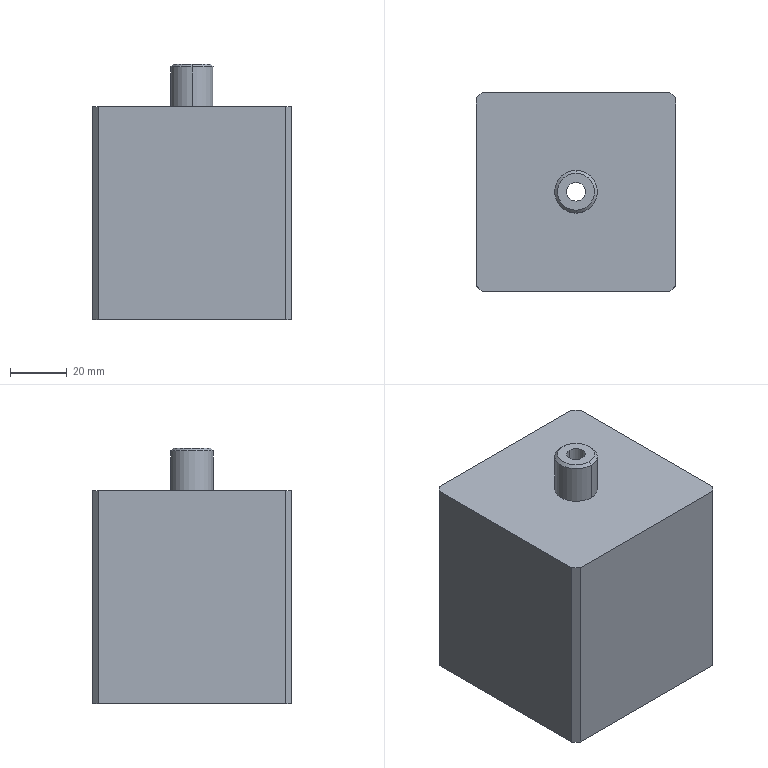NC program | NX | posted with a generic post | part box 70 x 70 x 90 mm
Lines 1 to 106 of 10206:
N10 G17 G21 G94 G90
(FLOOR_WALL_COPY , TOOL : D63)
N12 T01 M6
N14 G54
N16 G17 G0 G90 X-69.5 Y34.997 S6500 M3
N18 G43 Z30. H1
N20 Z10.
N22 G94 G1 Z7. F2500.
N24 X-66.5
N26 X66.5
N28 Y12.599
N30 X-66.5
N32 Y-9.8
N34 X66.5
N36 X69.5
N38 Z10.
N40 G0 Z30.
N42 X-69.5 Y34.997
N44 Z9.
N46 G1 Z6.
N48 X-66.5
N50 X66.5
N52 Y12.599
N54 X-66.5
N56 Y-9.8
N58 X66.5
N60 X69.5
N62 Z9.
N64 G0 Z30.
N66 X-69.5 Y34.997
N68 Z8.
N70 G1 Z5.
N72 X-66.5
N74 X66.5
N76 Y12.599
N78 X-66.5
N80 Y-9.8
N82 X66.5
N84 X69.5
N86 Z8.
N88 G0 Z30.
N90 X-69.5 Y34.997
N92 Z7.
N94 G1 Z4.
N96 X-66.5
N98 X66.5
N100 Y12.599
N102 X-66.5
N104 Y-9.8
N106 X66.5
N108 X69.5
N110 Z7.
N112 G0 Z30.
N114 X-69.5 Y34.997
N116 Z6.
N118 G1 Z3.
N120 X-66.5
N122 X66.5
N124 Y12.599
N126 X-66.5
N128 Y-9.8
N130 X66.5
N132 X69.5
N134 Z6.
N136 G0 Z30.
N138 X-69.5 Y34.997
N140 Z5.
N142 G1 Z2.
N144 X-66.5
N146 X66.5
N148 Y12.599
N150 X-66.5
N152 Y-9.8
N154 X66.5
N156 X69.5
N158 Z5.
N160 G0 Z30.
N162 X-69.5 Y34.997
N164 Z4.
N166 G1 Z1.
N168 X-66.5
N170 X66.5
N172 Y12.599
N174 X-66.5
N176 Y-9.8
N178 X66.5
N180 X69.5
N182 Z4.
N184 G0 Z30.
N186 X-69.5 Y34.997
N188 Z3.
N190 G1 Z0.
N192 X-66.5
N194 X66.5
N196 Y12.599
N198 X-66.5
N200 Y-9.8
N202 X66.5
N204 X69.5
N206 Z3.
N208 G0 Z30.
N210 M5